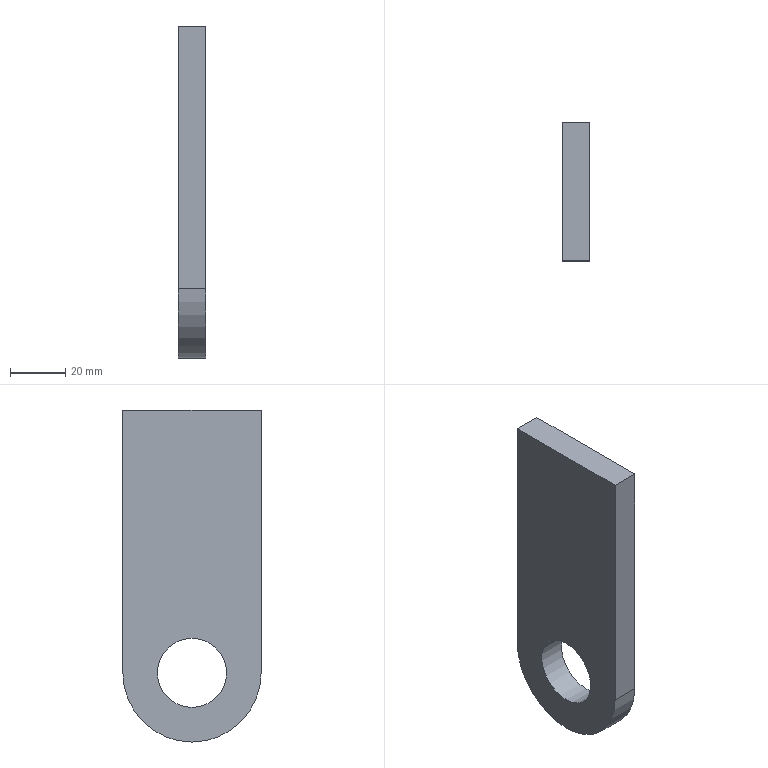Part | STEP file | subframe tilt hinge plate--000.001--20240928 | 1 solid | 7 faces | box 10 x 50 x 120 mm | volume 52409 mm3 | plane 5 | cylinder 2 | commonest cylinder face diameters 25 x1 50 x1
STEP:
#1=CARTESIAN_POINT('',(0.,0.,0.));
#2=DIRECTION('',(0.,0.,1.));
#3=DIRECTION('',(1.,0.,0.));
#4=AXIS2_PLACEMENT_3D('',#1,#2,#3);
#5=CARTESIAN_POINT('',(20.,393.5,0.));
#6=VERTEX_POINT('',#5);
#7=CARTESIAN_POINT('',(10.,393.5,0.));
#8=VERTEX_POINT('',#7);
#9=CARTESIAN_POINT('',(15.,393.5,0.));
#10=DIRECTION('',(-1.,0.,0.));
#11=VECTOR('',#10,1.);
#12=LINE('',#9,#11);
#13=CARTESIAN_POINT('',(-10.,490.,0.));
#14=DIRECTION('',(0.,0.,1.));
#15=DIRECTION('',(0.,-1.,0.));
#16=AXIS2_PLACEMENT_3D('',#13,#14,#15);
#17=PLANE('',#16);
#18=CARTESIAN_POINT('',(96.5,25.));
#19=DIRECTION('',(0.,-1.));
#20=VECTOR('',#19,1.);
#21=LINE('',#18,#20);
#22=(GEOMETRIC_REPRESENTATION_CONTEXT(2)PARAMETRIC_REPRESENTATION_CONTEXT()REPRESENTATION_CONTEXT('',''));
#23=DEFINITIONAL_REPRESENTATION('',(#21),#22);
#24=PCURVE('',#17,#23);
#25=CARTESIAN_POINT('',(15.,393.5,-130.));
#26=DIRECTION('',(0.,-1.,0.));
#27=DIRECTION('',(0.,0.,1.));
#28=AXIS2_PLACEMENT_3D('',#25,#26,#27);
#29=PLANE('',#28);
#30=CARTESIAN_POINT('',(130.,0.));
#31=DIRECTION('',(0.,1.));
#32=VECTOR('',#31,1.);
#33=LINE('',#30,#32);
#34=(GEOMETRIC_REPRESENTATION_CONTEXT(2)PARAMETRIC_REPRESENTATION_CONTEXT()REPRESENTATION_CONTEXT('',''));
#35=DEFINITIONAL_REPRESENTATION('',(#33),#34);
#36=PCURVE('',#29,#35);
#37=SURFACE_CURVE('',#12,(#24,#36),.PCURVE_S1.);
#38=EDGE_CURVE('',#6,#8,#37,.T.);
#39=ORIENTED_EDGE('',*,*,#38,.F.);
#40=CARTESIAN_POINT('',(20.,443.5,0.));
#41=VERTEX_POINT('',#40);
#42=CARTESIAN_POINT('',(20.,418.5,0.));
#43=DIRECTION('',(0.,-1.,0.));
#44=VECTOR('',#43,1.);
#45=LINE('',#42,#44);
#46=CARTESIAN_POINT('',(71.5,30.));
#47=DIRECTION('',(1.,0.));
#48=VECTOR('',#47,1.);
#49=LINE('',#46,#48);
#50=(GEOMETRIC_REPRESENTATION_CONTEXT(2)PARAMETRIC_REPRESENTATION_CONTEXT()REPRESENTATION_CONTEXT('',''));
#51=DEFINITIONAL_REPRESENTATION('',(#49),#50);
#52=PCURVE('',#17,#51);
#53=CARTESIAN_POINT('',(20.,418.5,-130.));
#54=DIRECTION('',(1.,0.,0.));
#55=DIRECTION('',(0.,0.,1.));
#56=AXIS2_PLACEMENT_3D('',#53,#54,#55);
#57=PLANE('',#56);
#58=CARTESIAN_POINT('',(130.,0.));
#59=DIRECTION('',(0.,1.));
#60=VECTOR('',#59,1.);
#61=LINE('',#58,#60);
#62=(GEOMETRIC_REPRESENTATION_CONTEXT(2)PARAMETRIC_REPRESENTATION_CONTEXT()REPRESENTATION_CONTEXT('',''));
#63=DEFINITIONAL_REPRESENTATION('',(#61),#62);
#64=PCURVE('',#57,#63);
#65=SURFACE_CURVE('',#45,(#52,#64),.PCURVE_S1.);
#66=EDGE_CURVE('',#41,#6,#65,.T.);
#67=ORIENTED_EDGE('',*,*,#66,.F.);
#68=CARTESIAN_POINT('',(10.,443.5,0.));
#69=VERTEX_POINT('',#68);
#70=CARTESIAN_POINT('',(15.,443.5,0.));
#71=DIRECTION('',(1.,0.,0.));
#72=VECTOR('',#71,1.);
#73=LINE('',#70,#72);
#74=CARTESIAN_POINT('',(46.5,25.));
#75=DIRECTION('',(0.,1.));
#76=VECTOR('',#75,1.);
#77=LINE('',#74,#76);
#78=(GEOMETRIC_REPRESENTATION_CONTEXT(2)PARAMETRIC_REPRESENTATION_CONTEXT()REPRESENTATION_CONTEXT('',''));
#79=DEFINITIONAL_REPRESENTATION('',(#77),#78);
#80=PCURVE('',#17,#79);
#81=CARTESIAN_POINT('',(15.,443.5,-130.));
#82=DIRECTION('',(0.,1.,0.));
#83=DIRECTION('',(0.,0.,-1.));
#84=AXIS2_PLACEMENT_3D('',#81,#82,#83);
#85=PLANE('',#84);
#86=CARTESIAN_POINT('',(-130.,0.));
#87=DIRECTION('',(0.,-1.));
#88=VECTOR('',#87,1.);
#89=LINE('',#86,#88);
#90=(GEOMETRIC_REPRESENTATION_CONTEXT(2)PARAMETRIC_REPRESENTATION_CONTEXT()REPRESENTATION_CONTEXT('',''));
#91=DEFINITIONAL_REPRESENTATION('',(#89),#90);
#92=PCURVE('',#85,#91);
#93=SURFACE_CURVE('',#73,(#80,#92),.PCURVE_S1.);
#94=EDGE_CURVE('',#69,#41,#93,.T.);
#95=ORIENTED_EDGE('',*,*,#94,.F.);
#96=CARTESIAN_POINT('',(10.,418.5,0.));
#97=DIRECTION('',(0.,1.,0.));
#98=VECTOR('',#97,1.);
#99=LINE('',#96,#98);
#100=CARTESIAN_POINT('',(71.5,20.));
#101=DIRECTION('',(-1.,0.));
#102=VECTOR('',#101,1.);
#103=LINE('',#100,#102);
#104=(GEOMETRIC_REPRESENTATION_CONTEXT(2)PARAMETRIC_REPRESENTATION_CONTEXT()REPRESENTATION_CONTEXT('',''));
#105=DEFINITIONAL_REPRESENTATION('',(#103),#104);
#106=PCURVE('',#17,#105);
#107=CARTESIAN_POINT('',(10.,418.5,-130.));
#108=DIRECTION('',(-1.,0.,0.));
#109=DIRECTION('',(0.,0.,-1.));
#110=AXIS2_PLACEMENT_3D('',#107,#108,#109);
#111=PLANE('',#110);
#112=CARTESIAN_POINT('',(-130.,0.));
#113=DIRECTION('',(0.,-1.));
#114=VECTOR('',#113,1.);
#115=LINE('',#112,#114);
#116=(GEOMETRIC_REPRESENTATION_CONTEXT(2)PARAMETRIC_REPRESENTATION_CONTEXT()REPRESENTATION_CONTEXT('',''));
#117=DEFINITIONAL_REPRESENTATION('',(#115),#116);
#118=PCURVE('',#111,#117);
#119=SURFACE_CURVE('',#99,(#106,#118),.PCURVE_S1.);
#120=EDGE_CURVE('',#8,#69,#119,.T.);
#121=ORIENTED_EDGE('',*,*,#120,.F.);
#122=EDGE_LOOP('',(#39,#67,#95,#121));
#123=FACE_BOUND('',#122,.T.);
#124=ADVANCED_FACE('',(#123),#17,.T.);
#125=CARTESIAN_POINT('',(10.,393.5,-95.));
#126=VERTEX_POINT('',#125);
#127=CARTESIAN_POINT('',(10.,393.5,-130.));
#128=DIRECTION('',(0.,0.,1.));
#129=VECTOR('',#128,1.);
#130=LINE('',#127,#129);
#131=CARTESIAN_POINT('',(0.,5.));
#132=DIRECTION('',(1.,0.));
#133=VECTOR('',#132,1.);
#134=LINE('',#131,#133);
#135=(GEOMETRIC_REPRESENTATION_CONTEXT(2)PARAMETRIC_REPRESENTATION_CONTEXT()REPRESENTATION_CONTEXT('',''));
#136=DEFINITIONAL_REPRESENTATION('',(#134),#135);
#137=PCURVE('',#29,#136);
#138=CARTESIAN_POINT('',(0.,25.));
#139=DIRECTION('',(-1.,0.));
#140=VECTOR('',#139,1.);
#141=LINE('',#138,#140);
#142=(GEOMETRIC_REPRESENTATION_CONTEXT(2)PARAMETRIC_REPRESENTATION_CONTEXT()REPRESENTATION_CONTEXT('',''));
#143=DEFINITIONAL_REPRESENTATION('',(#141),#142);
#144=PCURVE('',#111,#143);
#145=SURFACE_CURVE('',#130,(#137,#144),.PCURVE_S1.);
#146=EDGE_CURVE('',#126,#8,#145,.T.);
#147=ORIENTED_EDGE('',*,*,#146,.F.);
#148=CARTESIAN_POINT('',(20.,393.5,-95.));
#149=VERTEX_POINT('',#148);
#150=CARTESIAN_POINT('',(15.,393.5,-95.));
#151=DIRECTION('',(1.,0.,0.));
#152=VECTOR('',#151,1.);
#153=LINE('',#150,#152);
#154=CARTESIAN_POINT('',(35.,0.));
#155=DIRECTION('',(0.,-1.));
#156=VECTOR('',#155,1.);
#157=LINE('',#154,#156);
#158=(GEOMETRIC_REPRESENTATION_CONTEXT(2)PARAMETRIC_REPRESENTATION_CONTEXT()REPRESENTATION_CONTEXT('',''));
#159=DEFINITIONAL_REPRESENTATION('',(#157),#158);
#160=PCURVE('',#29,#159);
#161=CARTESIAN_POINT('',(15.,418.5,-95.));
#162=DIRECTION('',(-1.,0.,0.));
#163=DIRECTION('',(0.,0.,-1.));
#164=AXIS2_PLACEMENT_3D('',#161,#162,#163);
#165=CYLINDRICAL_SURFACE('',#164,25.);
#166=CARTESIAN_POINT('',(1.571,0.));
#167=DIRECTION('',(0.,-1.));
#168=VECTOR('',#167,1.);
#169=LINE('',#166,#168);
#170=(GEOMETRIC_REPRESENTATION_CONTEXT(2)PARAMETRIC_REPRESENTATION_CONTEXT()REPRESENTATION_CONTEXT('',''));
#171=DEFINITIONAL_REPRESENTATION('',(#169),#170);
#172=PCURVE('',#165,#171);
#173=SURFACE_CURVE('',#153,(#160,#172),.PCURVE_S1.);
#174=EDGE_CURVE('',#126,#149,#173,.T.);
#175=ORIENTED_EDGE('',*,*,#174,.T.);
#176=CARTESIAN_POINT('',(20.,393.5,-130.));
#177=DIRECTION('',(0.,0.,1.));
#178=VECTOR('',#177,1.);
#179=LINE('',#176,#178);
#180=CARTESIAN_POINT('',(0.,-5.));
#181=DIRECTION('',(1.,0.));
#182=VECTOR('',#181,1.);
#183=LINE('',#180,#182);
#184=(GEOMETRIC_REPRESENTATION_CONTEXT(2)PARAMETRIC_REPRESENTATION_CONTEXT()REPRESENTATION_CONTEXT('',''));
#185=DEFINITIONAL_REPRESENTATION('',(#183),#184);
#186=PCURVE('',#29,#185);
#187=CARTESIAN_POINT('',(0.,25.));
#188=DIRECTION('',(1.,0.));
#189=VECTOR('',#188,1.);
#190=LINE('',#187,#189);
#191=(GEOMETRIC_REPRESENTATION_CONTEXT(2)PARAMETRIC_REPRESENTATION_CONTEXT()REPRESENTATION_CONTEXT('',''));
#192=DEFINITIONAL_REPRESENTATION('',(#190),#191);
#193=PCURVE('',#57,#192);
#194=SURFACE_CURVE('',#179,(#186,#193),.PCURVE_S1.);
#195=EDGE_CURVE('',#149,#6,#194,.T.);
#196=ORIENTED_EDGE('',*,*,#195,.T.);
#197=ORIENTED_EDGE('',*,*,#38,.T.);
#198=EDGE_LOOP('',(#147,#175,#196,#197));
#199=FACE_BOUND('',#198,.T.);
#200=ADVANCED_FACE('',(#199),#29,.T.);
#201=CARTESIAN_POINT('',(10.,418.5,-82.5));
#202=VERTEX_POINT('',#201);
#203=CARTESIAN_POINT('',(10.,418.5,-107.5));
#204=VERTEX_POINT('',#203);
#205=CARTESIAN_POINT('',(10.,418.5,-95.));
#206=DIRECTION('',(1.,0.,0.));
#207=DIRECTION('',(0.,0.,1.));
#208=AXIS2_PLACEMENT_3D('',#205,#206,#207);
#209=CIRCLE('',#208,12.5);
#210=CARTESIAN_POINT('',(-47.5,0.));
#211=CARTESIAN_POINT('',(-47.5,21.651));
#212=CARTESIAN_POINT('',(-28.75,10.825));
#213=CARTESIAN_POINT('',(-10.,0.));
#214=CARTESIAN_POINT('',(-28.75,-10.825));
#215=CARTESIAN_POINT('',(-47.5,-21.651));
#216=CARTESIAN_POINT('',(-47.5,0.));
#217=(BOUNDED_CURVE()B_SPLINE_CURVE(2,(#210,#211,#212,#213,#214,#215,#216),.UNSPECIFIED.,.T.,.F.)B_SPLINE_CURVE_WITH_KNOTS((1,2,2,2,2,1),(-2.094,0.,2.094,4.189,6.283,8.378),.UNSPECIFIED.)CURVE()GEOMETRIC_REPRESENTATION_ITEM()RATIONAL_B_SPLINE_CURVE((1.,0.5,1.,0.5,1.,0.5,1.))REPRESENTATION_ITEM(''));
#218=(GEOMETRIC_REPRESENTATION_CONTEXT(2)PARAMETRIC_REPRESENTATION_CONTEXT()REPRESENTATION_CONTEXT('',''));
#219=DEFINITIONAL_REPRESENTATION('',(#217),#218);
#220=PCURVE('',#111,#219);
#221=CARTESIAN_POINT('',(-30.,418.5,-95.));
#222=DIRECTION('',(1.,0.,0.));
#223=DIRECTION('',(0.,-1.,0.));
#224=AXIS2_PLACEMENT_3D('',#221,#222,#223);
#225=CYLINDRICAL_SURFACE('',#224,12.5);
#226=CARTESIAN_POINT('',(4.712,40.));
#227=DIRECTION('',(1.,0.));
#228=VECTOR('',#227,1.);
#229=LINE('',#226,#228);
#230=(GEOMETRIC_REPRESENTATION_CONTEXT(2)PARAMETRIC_REPRESENTATION_CONTEXT()REPRESENTATION_CONTEXT('',''));
#231=DEFINITIONAL_REPRESENTATION('',(#229),#230);
#232=PCURVE('',#225,#231);
#233=SURFACE_CURVE('',#209,(#220,#232),.PCURVE_S1.);
#234=EDGE_CURVE('',#202,#204,#233,.T.);
#235=ORIENTED_EDGE('',*,*,#234,.T.);
#236=CARTESIAN_POINT('',(10.,418.5,-95.));
#237=DIRECTION('',(1.,0.,0.));
#238=DIRECTION('',(0.,0.,1.));
#239=AXIS2_PLACEMENT_3D('',#236,#237,#238);
#240=CIRCLE('',#239,12.5);
#241=CARTESIAN_POINT('',(-47.5,0.));
#242=CARTESIAN_POINT('',(-47.5,21.651));
#243=CARTESIAN_POINT('',(-28.75,10.825));
#244=CARTESIAN_POINT('',(-10.,0.));
#245=CARTESIAN_POINT('',(-28.75,-10.825));
#246=CARTESIAN_POINT('',(-47.5,-21.651));
#247=CARTESIAN_POINT('',(-47.5,0.));
#248=(BOUNDED_CURVE()B_SPLINE_CURVE(2,(#241,#242,#243,#244,#245,#246,#247),.UNSPECIFIED.,.T.,.F.)B_SPLINE_CURVE_WITH_KNOTS((1,2,2,2,2,1),(-2.094,0.,2.094,4.189,6.283,8.378),.UNSPECIFIED.)CURVE()GEOMETRIC_REPRESENTATION_ITEM()RATIONAL_B_SPLINE_CURVE((1.,0.5,1.,0.5,1.,0.5,1.))REPRESENTATION_ITEM(''));
#249=(GEOMETRIC_REPRESENTATION_CONTEXT(2)PARAMETRIC_REPRESENTATION_CONTEXT()REPRESENTATION_CONTEXT('',''));
#250=DEFINITIONAL_REPRESENTATION('',(#248),#249);
#251=PCURVE('',#111,#250);
#252=CARTESIAN_POINT('',(-1.571,40.));
#253=DIRECTION('',(1.,0.));
#254=VECTOR('',#253,1.);
#255=LINE('',#252,#254);
#256=(GEOMETRIC_REPRESENTATION_CONTEXT(2)PARAMETRIC_REPRESENTATION_CONTEXT()REPRESENTATION_CONTEXT('',''));
#257=DEFINITIONAL_REPRESENTATION('',(#255),#256);
#258=PCURVE('',#225,#257);
#259=SURFACE_CURVE('',#240,(#251,#258),.PCURVE_S1.);
#260=EDGE_CURVE('',#204,#202,#259,.T.);
#261=ORIENTED_EDGE('',*,*,#260,.T.);
#262=EDGE_LOOP('',(#235,#261));
#263=FACE_BOUND('',#262,.T.);
#264=CARTESIAN_POINT('',(10.,443.5,-95.));
#265=VERTEX_POINT('',#264);
#266=CARTESIAN_POINT('',(10.,418.5,-95.));
#267=DIRECTION('',(-1.,0.,0.));
#268=DIRECTION('',(0.,0.,1.));
#269=AXIS2_PLACEMENT_3D('',#266,#267,#268);
#270=CIRCLE('',#269,25.);
#271=CARTESIAN_POINT('',(-35.,0.));
#272=DIRECTION('',(-1.,0.));
#273=AXIS2_PLACEMENT_2D('',#271,#272);
#274=CIRCLE('',#273,25.);
#275=(GEOMETRIC_REPRESENTATION_CONTEXT(2)PARAMETRIC_REPRESENTATION_CONTEXT()REPRESENTATION_CONTEXT('',''));
#276=DEFINITIONAL_REPRESENTATION('',(#274),#275);
#277=PCURVE('',#111,#276);
#278=CARTESIAN_POINT('',(-3.142,5.));
#279=DIRECTION('',(1.,0.));
#280=VECTOR('',#279,1.);
#281=LINE('',#278,#280);
#282=(GEOMETRIC_REPRESENTATION_CONTEXT(2)PARAMETRIC_REPRESENTATION_CONTEXT()REPRESENTATION_CONTEXT('',''));
#283=DEFINITIONAL_REPRESENTATION('',(#281),#282);
#284=PCURVE('',#165,#283);
#285=SURFACE_CURVE('',#270,(#277,#284),.PCURVE_S1.);
#286=EDGE_CURVE('',#265,#126,#285,.T.);
#287=ORIENTED_EDGE('',*,*,#286,.T.);
#288=ORIENTED_EDGE('',*,*,#146,.T.);
#289=ORIENTED_EDGE('',*,*,#120,.T.);
#290=CARTESIAN_POINT('',(10.,443.5,-130.));
#291=DIRECTION('',(0.,0.,1.));
#292=VECTOR('',#291,1.);
#293=LINE('',#290,#292);
#294=CARTESIAN_POINT('',(0.,-25.));
#295=DIRECTION('',(-1.,0.));
#296=VECTOR('',#295,1.);
#297=LINE('',#294,#296);
#298=(GEOMETRIC_REPRESENTATION_CONTEXT(2)PARAMETRIC_REPRESENTATION_CONTEXT()REPRESENTATION_CONTEXT('',''));
#299=DEFINITIONAL_REPRESENTATION('',(#297),#298);
#300=PCURVE('',#111,#299);
#301=CARTESIAN_POINT('',(0.,5.));
#302=DIRECTION('',(-1.,0.));
#303=VECTOR('',#302,1.);
#304=LINE('',#301,#303);
#305=(GEOMETRIC_REPRESENTATION_CONTEXT(2)PARAMETRIC_REPRESENTATION_CONTEXT()REPRESENTATION_CONTEXT('',''));
#306=DEFINITIONAL_REPRESENTATION('',(#304),#305);
#307=PCURVE('',#85,#306);
#308=SURFACE_CURVE('',#293,(#300,#307),.PCURVE_S1.);
#309=EDGE_CURVE('',#265,#69,#308,.T.);
#310=ORIENTED_EDGE('',*,*,#309,.F.);
#311=EDGE_LOOP('',(#287,#288,#289,#310));
#312=FACE_BOUND('',#311,.T.);
#313=ADVANCED_FACE('',(#263,#312),#111,.T.);
#314=CARTESIAN_POINT('',(20.,443.5,-95.));
#315=VERTEX_POINT('',#314);
#316=CARTESIAN_POINT('',(20.,443.5,-130.));
#317=DIRECTION('',(0.,0.,1.));
#318=VECTOR('',#317,1.);
#319=LINE('',#316,#318);
#320=CARTESIAN_POINT('',(0.,-5.));
#321=DIRECTION('',(-1.,0.));
#322=VECTOR('',#321,1.);
#323=LINE('',#320,#322);
#324=(GEOMETRIC_REPRESENTATION_CONTEXT(2)PARAMETRIC_REPRESENTATION_CONTEXT()REPRESENTATION_CONTEXT('',''));
#325=DEFINITIONAL_REPRESENTATION('',(#323),#324);
#326=PCURVE('',#85,#325);
#327=CARTESIAN_POINT('',(0.,-25.));
#328=DIRECTION('',(1.,0.));
#329=VECTOR('',#328,1.);
#330=LINE('',#327,#329);
#331=(GEOMETRIC_REPRESENTATION_CONTEXT(2)PARAMETRIC_REPRESENTATION_CONTEXT()REPRESENTATION_CONTEXT('',''));
#332=DEFINITIONAL_REPRESENTATION('',(#330),#331);
#333=PCURVE('',#57,#332);
#334=SURFACE_CURVE('',#319,(#326,#333),.PCURVE_S1.);
#335=EDGE_CURVE('',#315,#41,#334,.T.);
#336=ORIENTED_EDGE('',*,*,#335,.F.);
#337=CARTESIAN_POINT('',(15.,443.5,-95.));
#338=DIRECTION('',(-1.,0.,0.));
#339=VECTOR('',#338,1.);
#340=LINE('',#337,#339);
#341=CARTESIAN_POINT('',(-35.,0.));
#342=DIRECTION('',(0.,1.));
#343=VECTOR('',#342,1.);
#344=LINE('',#341,#343);
#345=(GEOMETRIC_REPRESENTATION_CONTEXT(2)PARAMETRIC_REPRESENTATION_CONTEXT()REPRESENTATION_CONTEXT('',''));
#346=DEFINITIONAL_REPRESENTATION('',(#344),#345);
#347=PCURVE('',#85,#346);
#348=CARTESIAN_POINT('',(-1.571,0.));
#349=DIRECTION('',(0.,1.));
#350=VECTOR('',#349,1.);
#351=LINE('',#348,#350);
#352=(GEOMETRIC_REPRESENTATION_CONTEXT(2)PARAMETRIC_REPRESENTATION_CONTEXT()REPRESENTATION_CONTEXT('',''));
#353=DEFINITIONAL_REPRESENTATION('',(#351),#352);
#354=PCURVE('',#165,#353);
#355=SURFACE_CURVE('',#340,(#347,#354),.PCURVE_S1.);
#356=EDGE_CURVE('',#315,#265,#355,.T.);
#357=ORIENTED_EDGE('',*,*,#356,.T.);
#358=ORIENTED_EDGE('',*,*,#309,.T.);
#359=ORIENTED_EDGE('',*,*,#94,.T.);
#360=EDGE_LOOP('',(#336,#357,#358,#359));
#361=FACE_BOUND('',#360,.T.);
#362=ADVANCED_FACE('',(#361),#85,.T.);
#363=CARTESIAN_POINT('',(20.,418.5,-107.5));
#364=VERTEX_POINT('',#363);
#365=CARTESIAN_POINT('',(20.,418.5,-95.));
#366=DIRECTION('',(-1.,0.,0.));
#367=DIRECTION('',(0.,0.,-1.));
#368=AXIS2_PLACEMENT_3D('',#365,#366,#367);
#369=CIRCLE('',#368,12.5);
#370=CARTESIAN_POINT('',(22.5,0.));
#371=CARTESIAN_POINT('',(22.5,21.651));
#372=CARTESIAN_POINT('',(41.25,10.825));
#373=CARTESIAN_POINT('',(60.,0.));
#374=CARTESIAN_POINT('',(41.25,-10.825));
#375=CARTESIAN_POINT('',(22.5,-21.651));
#376=CARTESIAN_POINT('',(22.5,0.));
#377=(BOUNDED_CURVE()B_SPLINE_CURVE(2,(#370,#371,#372,#373,#374,#375,#376),.UNSPECIFIED.,.T.,.F.)B_SPLINE_CURVE_WITH_KNOTS((1,2,2,2,2,1),(-2.094,0.,2.094,4.189,6.283,8.378),.UNSPECIFIED.)CURVE()GEOMETRIC_REPRESENTATION_ITEM()RATIONAL_B_SPLINE_CURVE((1.,0.5,1.,0.5,1.,0.5,1.))REPRESENTATION_ITEM(''));
#378=(GEOMETRIC_REPRESENTATION_CONTEXT(2)PARAMETRIC_REPRESENTATION_CONTEXT()REPRESENTATION_CONTEXT('',''));
#379=DEFINITIONAL_REPRESENTATION('',(#377),#378);
#380=PCURVE('',#57,#379);
#381=CARTESIAN_POINT('',(7.854,50.));
#382=DIRECTION('',(-1.,0.));
#383=VECTOR('',#382,1.);
#384=LINE('',#381,#383);
#385=(GEOMETRIC_REPRESENTATION_CONTEXT(2)PARAMETRIC_REPRESENTATION_CONTEXT()REPRESENTATION_CONTEXT('',''));
#386=DEFINITIONAL_REPRESENTATION('',(#384),#385);
#387=PCURVE('',#225,#386);
#388=SURFACE_CURVE('',#369,(#380,#387),.PCURVE_S1.);
#389=EDGE_CURVE('',#364,#364,#388,.T.);
#390=ORIENTED_EDGE('',*,*,#389,.T.);
#391=EDGE_LOOP('',(#390));
#392=FACE_BOUND('',#391,.T.);
#393=ORIENTED_EDGE('',*,*,#195,.F.);
#394=CARTESIAN_POINT('',(20.,418.5,-95.));
#395=DIRECTION('',(1.,0.,0.));
#396=DIRECTION('',(0.,0.,-1.));
#397=AXIS2_PLACEMENT_3D('',#394,#395,#396);
#398=CIRCLE('',#397,25.);
#399=CARTESIAN_POINT('',(35.,0.));
#400=DIRECTION('',(-1.,0.));
#401=AXIS2_PLACEMENT_2D('',#399,#400);
#402=CIRCLE('',#401,25.);
#403=(GEOMETRIC_REPRESENTATION_CONTEXT(2)PARAMETRIC_REPRESENTATION_CONTEXT()REPRESENTATION_CONTEXT('',''));
#404=DEFINITIONAL_REPRESENTATION('',(#402),#403);
#405=PCURVE('',#57,#404);
#406=CARTESIAN_POINT('',(6.283,-5.));
#407=DIRECTION('',(-1.,0.));
#408=VECTOR('',#407,1.);
#409=LINE('',#406,#408);
#410=(GEOMETRIC_REPRESENTATION_CONTEXT(2)PARAMETRIC_REPRESENTATION_CONTEXT()REPRESENTATION_CONTEXT('',''));
#411=DEFINITIONAL_REPRESENTATION('',(#409),#410);
#412=PCURVE('',#165,#411);
#413=SURFACE_CURVE('',#398,(#405,#412),.PCURVE_S1.);
#414=EDGE_CURVE('',#149,#315,#413,.T.);
#415=ORIENTED_EDGE('',*,*,#414,.T.);
#416=ORIENTED_EDGE('',*,*,#335,.T.);
#417=ORIENTED_EDGE('',*,*,#66,.T.);
#418=EDGE_LOOP('',(#393,#415,#416,#417));
#419=FACE_BOUND('',#418,.T.);
#420=ADVANCED_FACE('',(#392,#419),#57,.T.);
#421=ORIENTED_EDGE('',*,*,#389,.T.);
#422=CARTESIAN_POINT('',(10.,418.5,-107.5));
#423=CARTESIAN_POINT('',(20.,418.5,-107.5));
#424=B_SPLINE_CURVE_WITH_KNOTS('',1,(#422,#423),.UNSPECIFIED.,.F.,.F.,(2,2),(40.,50.),.PIECEWISE_BEZIER_KNOTS.);
#425=CARTESIAN_POINT('',(1.571,0.));
#426=DIRECTION('',(0.,1.));
#427=VECTOR('',#426,1.);
#428=LINE('',#425,#427);
#429=(GEOMETRIC_REPRESENTATION_CONTEXT(2)PARAMETRIC_REPRESENTATION_CONTEXT()REPRESENTATION_CONTEXT('',''));
#430=DEFINITIONAL_REPRESENTATION('',(#428),#429);
#431=PCURVE('',#225,#430);
#432=CARTESIAN_POINT('',(7.854,0.));
#433=DIRECTION('',(0.,1.));
#434=VECTOR('',#433,1.);
#435=LINE('',#432,#434);
#436=(GEOMETRIC_REPRESENTATION_CONTEXT(2)PARAMETRIC_REPRESENTATION_CONTEXT()REPRESENTATION_CONTEXT('',''));
#437=DEFINITIONAL_REPRESENTATION('',(#435),#436);
#438=PCURVE('',#225,#437);
#439=SEAM_CURVE('',#424,(#431,#438),.PCURVE_S1.);
#440=EDGE_CURVE('',#204,#364,#439,.T.);
#441=ORIENTED_EDGE('',*,*,#440,.F.);
#442=ORIENTED_EDGE('',*,*,#260,.T.);
#443=ORIENTED_EDGE('',*,*,#234,.T.);
#444=ORIENTED_EDGE('',*,*,#440,.T.);
#445=EDGE_LOOP('',(#421,#441,#442,#443,#444));
#446=FACE_BOUND('',#445,.F.);
#447=ADVANCED_FACE('',(#446),#225,.F.);
#448=ORIENTED_EDGE('',*,*,#414,.F.);
#449=ORIENTED_EDGE('',*,*,#174,.F.);
#450=ORIENTED_EDGE('',*,*,#286,.F.);
#451=ORIENTED_EDGE('',*,*,#356,.F.);
#452=EDGE_LOOP('',(#448,#449,#450,#451));
#453=FACE_BOUND('',#452,.T.);
#454=ADVANCED_FACE('',(#453),#165,.T.);
#455=CLOSED_SHELL('',(#124,#200,#313,#362,#420,#447,#454));
#456=MANIFOLD_SOLID_BREP('',#455);
#457=(LENGTH_UNIT()NAMED_UNIT(*)SI_UNIT(.MILLI.,.METRE.));
#458=UNCERTAINTY_MEASURE_WITH_UNIT(LENGTH_MEASURE(0.000002),#457,'','');
#459=(NAMED_UNIT(*)PLANE_ANGLE_UNIT()SI_UNIT($,.RADIAN.));
#460=(NAMED_UNIT(*)SI_UNIT($,.STERADIAN.)SOLID_ANGLE_UNIT());
#461=(GEOMETRIC_REPRESENTATION_CONTEXT(3)GLOBAL_UNCERTAINTY_ASSIGNED_CONTEXT((#458))GLOBAL_UNIT_ASSIGNED_CONTEXT((#457,#459,#460))REPRESENTATION_CONTEXT('',''));
#462=ADVANCED_BREP_SHAPE_REPRESENTATION('',(#4,#456),#461);